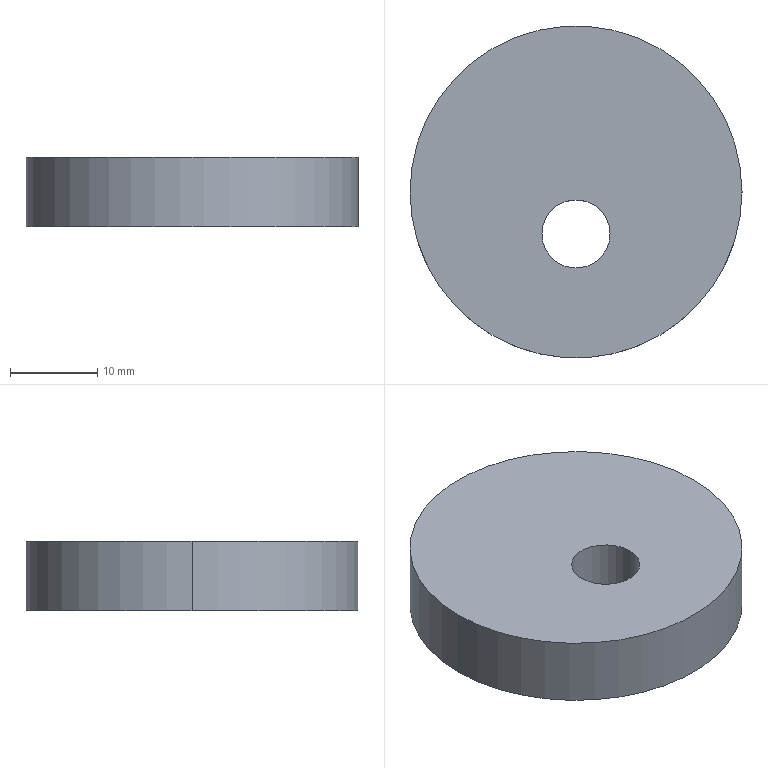Part | SolidWorks | features Extrusion 1 | 1 solid | 6 faces | box 38 x 38 x 8 mm | volume 8691 mm3 | cylinder 4 | plane 2 | commonest cylinder face diameters 7.8 x2 38 x2
STEP:
#1=CARTESIAN_POINT('',(-3.9,-74.77,4.));
#2=VERTEX_POINT('',#1);
#3=CARTESIAN_POINT('',(3.9,-74.77,4.));
#4=VERTEX_POINT('',#3);
#5=CARTESIAN_POINT('',(0.,-74.77,4.));
#6=DIRECTION('',(0.,0.,1.));
#7=DIRECTION('',(1.,0.,0.));
#8=AXIS2_PLACEMENT_3D('',#5,#6,#7);
#9=CIRCLE('',#8,3.9);
#10=EDGE_CURVE('',#2,#4,#9,.T.);
#11=ORIENTED_EDGE('',*,*,#10,.T.);
#12=CARTESIAN_POINT('',(3.9,-74.77,-4.));
#13=VERTEX_POINT('',#12);
#14=CARTESIAN_POINT('',(3.9,-74.77,4.));
#15=DIRECTION('',(0.,0.,-1.));
#16=VECTOR('',#15,1000.);
#17=LINE('',#14,#16);
#18=EDGE_CURVE('',#4,#13,#17,.T.);
#19=ORIENTED_EDGE('',*,*,#18,.T.);
#20=CARTESIAN_POINT('',(-3.9,-74.77,-4.));
#21=VERTEX_POINT('',#20);
#22=CARTESIAN_POINT('',(0.,-74.77,-4.));
#23=DIRECTION('',(0.,0.,1.));
#24=DIRECTION('',(1.,0.,0.));
#25=AXIS2_PLACEMENT_3D('',#22,#23,#24);
#26=CIRCLE('',#25,3.9);
#27=EDGE_CURVE('',#21,#13,#26,.T.);
#28=ORIENTED_EDGE('',*,*,#27,.F.);
#29=CARTESIAN_POINT('',(-3.9,-74.77,4.));
#30=DIRECTION('',(0.,0.,-1.));
#31=VECTOR('',#30,1000.);
#32=LINE('',#29,#31);
#33=EDGE_CURVE('',#2,#21,#32,.T.);
#34=ORIENTED_EDGE('',*,*,#33,.F.);
#35=EDGE_LOOP('',(#11,#19,#28,#34));
#36=FACE_OUTER_BOUND('',#35,.T.);
#37=CARTESIAN_POINT('',(0.,-74.77,4.));
#38=DIRECTION('',(0.,0.,-1.));
#39=DIRECTION('',(-1.,0.,0.));
#40=AXIS2_PLACEMENT_3D('',#37,#38,#39);
#41=CYLINDRICAL_SURFACE('',#40,3.9);
#42=ADVANCED_FACE('',(#36),#41,.F.);
#43=CARTESIAN_POINT('',(19.,-69.97,4.));
#44=VERTEX_POINT('',#43);
#45=CARTESIAN_POINT('',(-19.,-69.97,4.));
#46=VERTEX_POINT('',#45);
#47=CARTESIAN_POINT('',(0.,-69.97,4.));
#48=DIRECTION('',(0.,0.,1.));
#49=DIRECTION('',(1.,0.,0.));
#50=AXIS2_PLACEMENT_3D('',#47,#48,#49);
#51=CIRCLE('',#50,19.);
#52=EDGE_CURVE('',#44,#46,#51,.T.);
#53=ORIENTED_EDGE('',*,*,#52,.F.);
#54=CARTESIAN_POINT('',(19.,-69.97,-4.));
#55=VERTEX_POINT('',#54);
#56=CARTESIAN_POINT('',(19.,-69.97,4.));
#57=DIRECTION('',(0.,0.,-1.));
#58=VECTOR('',#57,1000.);
#59=LINE('',#56,#58);
#60=EDGE_CURVE('',#44,#55,#59,.T.);
#61=ORIENTED_EDGE('',*,*,#60,.T.);
#62=CARTESIAN_POINT('',(-19.,-69.97,-4.));
#63=VERTEX_POINT('',#62);
#64=CARTESIAN_POINT('',(0.,-69.97,-4.));
#65=DIRECTION('',(0.,0.,1.));
#66=DIRECTION('',(1.,0.,0.));
#67=AXIS2_PLACEMENT_3D('',#64,#65,#66);
#68=CIRCLE('',#67,19.);
#69=EDGE_CURVE('',#55,#63,#68,.T.);
#70=ORIENTED_EDGE('',*,*,#69,.T.);
#71=CARTESIAN_POINT('',(-19.,-69.97,4.));
#72=DIRECTION('',(0.,0.,-1.));
#73=VECTOR('',#72,1000.);
#74=LINE('',#71,#73);
#75=EDGE_CURVE('',#46,#63,#74,.T.);
#76=ORIENTED_EDGE('',*,*,#75,.F.);
#77=EDGE_LOOP('',(#53,#61,#70,#76));
#78=FACE_OUTER_BOUND('',#77,.T.);
#79=CARTESIAN_POINT('',(0.,-69.97,4.));
#80=DIRECTION('',(0.,0.,-1.));
#81=DIRECTION('',(-1.,0.,0.));
#82=AXIS2_PLACEMENT_3D('',#79,#80,#81);
#83=CYLINDRICAL_SURFACE('',#82,19.);
#84=ADVANCED_FACE('',(#78),#83,.T.);
#85=CARTESIAN_POINT('',(0.,-69.97,4.));
#86=DIRECTION('',(0.,0.,1.));
#87=DIRECTION('',(1.,0.,0.));
#88=AXIS2_PLACEMENT_3D('',#85,#86,#87);
#89=CIRCLE('',#88,19.);
#90=EDGE_CURVE('',#46,#44,#89,.T.);
#91=ORIENTED_EDGE('',*,*,#90,.T.);
#92=ORIENTED_EDGE('',*,*,#52,.T.);
#93=EDGE_LOOP('',(#91,#92));
#94=FACE_OUTER_BOUND('',#93,.T.);
#95=ORIENTED_EDGE('',*,*,#10,.F.);
#96=CARTESIAN_POINT('',(0.,-74.77,4.));
#97=DIRECTION('',(0.,0.,1.));
#98=DIRECTION('',(1.,0.,0.));
#99=AXIS2_PLACEMENT_3D('',#96,#97,#98);
#100=CIRCLE('',#99,3.9);
#101=EDGE_CURVE('',#4,#2,#100,.T.);
#102=ORIENTED_EDGE('',*,*,#101,.F.);
#103=EDGE_LOOP('',(#95,#102));
#104=FACE_BOUND('',#103,.T.);
#105=CARTESIAN_POINT('',(0.,-69.97,4.));
#106=DIRECTION('',(0.,0.,1.));
#107=DIRECTION('',(1.,0.,0.));
#108=AXIS2_PLACEMENT_3D('',#105,#106,#107);
#109=PLANE('',#108);
#110=ADVANCED_FACE('',(#94,#104),#109,.T.);
#111=CARTESIAN_POINT('',(0.,-69.97,-4.));
#112=DIRECTION('',(0.,0.,1.));
#113=DIRECTION('',(1.,0.,0.));
#114=AXIS2_PLACEMENT_3D('',#111,#112,#113);
#115=CIRCLE('',#114,19.);
#116=EDGE_CURVE('',#63,#55,#115,.T.);
#117=ORIENTED_EDGE('',*,*,#116,.F.);
#118=ORIENTED_EDGE('',*,*,#69,.F.);
#119=EDGE_LOOP('',(#117,#118));
#120=FACE_OUTER_BOUND('',#119,.T.);
#121=ORIENTED_EDGE('',*,*,#27,.T.);
#122=CARTESIAN_POINT('',(0.,-74.77,-4.));
#123=DIRECTION('',(0.,0.,1.));
#124=DIRECTION('',(1.,0.,0.));
#125=AXIS2_PLACEMENT_3D('',#122,#123,#124);
#126=CIRCLE('',#125,3.9);
#127=EDGE_CURVE('',#13,#21,#126,.T.);
#128=ORIENTED_EDGE('',*,*,#127,.T.);
#129=EDGE_LOOP('',(#121,#128));
#130=FACE_BOUND('',#129,.T.);
#131=CARTESIAN_POINT('',(0.,-69.97,-4.));
#132=DIRECTION('',(0.,0.,1.));
#133=DIRECTION('',(1.,0.,0.));
#134=AXIS2_PLACEMENT_3D('',#131,#132,#133);
#135=PLANE('',#134);
#136=ADVANCED_FACE('',(#120,#130),#135,.F.);
#137=ORIENTED_EDGE('',*,*,#60,.F.);
#138=ORIENTED_EDGE('',*,*,#90,.F.);
#139=ORIENTED_EDGE('',*,*,#75,.T.);
#140=ORIENTED_EDGE('',*,*,#116,.T.);
#141=EDGE_LOOP('',(#137,#138,#139,#140));
#142=FACE_OUTER_BOUND('',#141,.T.);
#143=CARTESIAN_POINT('',(0.,-69.97,4.));
#144=DIRECTION('',(0.,0.,-1.));
#145=DIRECTION('',(-1.,0.,0.));
#146=AXIS2_PLACEMENT_3D('',#143,#144,#145);
#147=CYLINDRICAL_SURFACE('',#146,19.);
#148=ADVANCED_FACE('',(#142),#147,.T.);
#149=ORIENTED_EDGE('',*,*,#18,.F.);
#150=ORIENTED_EDGE('',*,*,#101,.T.);
#151=ORIENTED_EDGE('',*,*,#33,.T.);
#152=ORIENTED_EDGE('',*,*,#127,.F.);
#153=EDGE_LOOP('',(#149,#150,#151,#152));
#154=FACE_OUTER_BOUND('',#153,.T.);
#155=CARTESIAN_POINT('',(0.,-74.77,4.));
#156=DIRECTION('',(0.,0.,-1.));
#157=DIRECTION('',(-1.,0.,0.));
#158=AXIS2_PLACEMENT_3D('',#155,#156,#157);
#159=CYLINDRICAL_SURFACE('',#158,3.9);
#160=ADVANCED_FACE('',(#154),#159,.F.);
#161=CLOSED_SHELL('',(#42,#84,#110,#136,#148,#160));
#162=MANIFOLD_SOLID_BREP('',#161);
#163=CARTESIAN_POINT('',(0.,0.,0.));
#164=DIRECTION('',(0.,0.,1.));
#165=DIRECTION('',(1.,0.,0.));
#166=AXIS2_PLACEMENT_3D('',#163,#164,#165);
#167=(LENGTH_UNIT()NAMED_UNIT(*)SI_UNIT(.MILLI.,.METRE.));
#168=UNCERTAINTY_MEASURE_WITH_UNIT(LENGTH_MEASURE(0.00001),#167,'','');
#169=(NAMED_UNIT(*)PLANE_ANGLE_UNIT()SI_UNIT($,.RADIAN.));
#170=(NAMED_UNIT(*)SI_UNIT($,.STERADIAN.)SOLID_ANGLE_UNIT());
#171=(GEOMETRIC_REPRESENTATION_CONTEXT(3)GLOBAL_UNCERTAINTY_ASSIGNED_CONTEXT((#168))GLOBAL_UNIT_ASSIGNED_CONTEXT((#167,#169,#170))REPRESENTATION_CONTEXT('',''));
#172=ADVANCED_BREP_SHAPE_REPRESENTATION('',(#162,#166),#171);